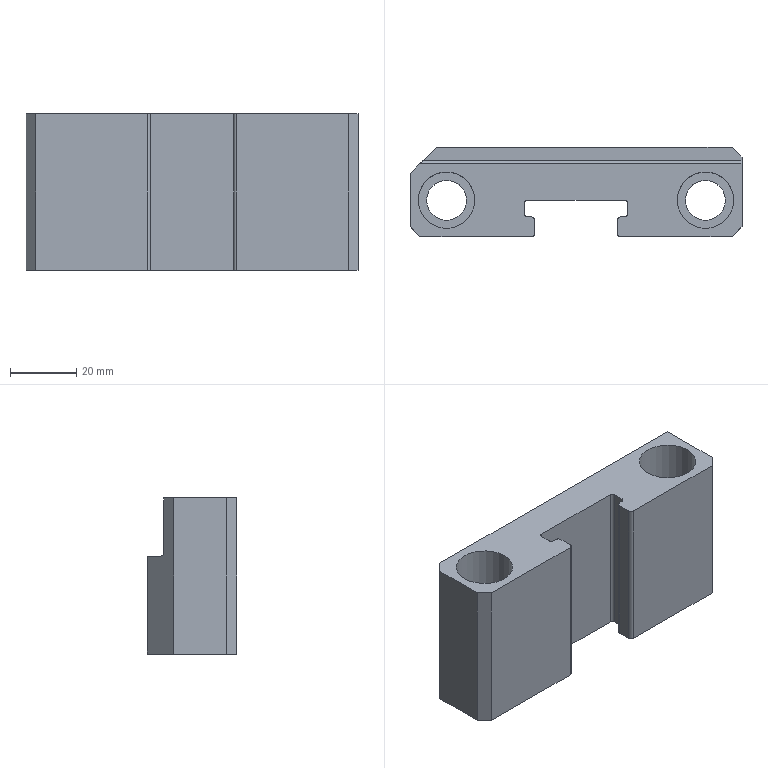Part | NX | features DIE-84 2 | 1 solid | 35 faces | box 100 x 27 x 47 mm | volume 84311 mm3 | plane 22 | cylinder 13 | commonest cylinder face diameters 1.8 x4 2 x3 2.2 x2 12.002 x2 17 x2
STEP:
#1=CARTESIAN_POINT('',(3996.095,-923.622,813.716));
#2=VERTEX_POINT('',#1);
#3=CARTESIAN_POINT('',(3990.094,-923.622,813.716));
#4=DIRECTION('',(0.,0.,1.));
#5=DIRECTION('',(1.,0.,0.));
#6=AXIS2_PLACEMENT_3D('',#3,#4,#5);
#7=CIRCLE('',#6,6.001);
#8=EDGE_CURVE('',#2,#2,#7,.T.);
#9=ORIENTED_EDGE('',*,*,#8,.T.);
#10=EDGE_LOOP('',(#9));
#11=FACE_BOUND('',#10,.T.);
#12=CARTESIAN_POINT('',(3906.093,-923.622,813.716));
#13=VERTEX_POINT('',#12);
#14=CARTESIAN_POINT('',(3912.094,-923.622,813.716));
#15=DIRECTION('',(0.,0.,-1.));
#16=DIRECTION('',(-1.,0.,0.));
#17=AXIS2_PLACEMENT_3D('',#14,#15,#16);
#18=CIRCLE('',#17,6.001);
#19=EDGE_CURVE('',#13,#13,#18,.T.);
#20=ORIENTED_EDGE('',*,*,#19,.F.);
#21=EDGE_LOOP('',(#20));
#22=FACE_BOUND('',#21,.T.);
#23=CARTESIAN_POINT('',(3964.599,-934.622,813.716));
#24=VERTEX_POINT('',#23);
#25=CARTESIAN_POINT('',(3998.094,-934.622,813.716));
#26=VERTEX_POINT('',#25);
#27=CARTESIAN_POINT('',(3911.094,-934.622,813.716));
#28=DIRECTION('',(1.,0.,0.));
#29=VECTOR('',#28,1000.);
#30=LINE('',#27,#29);
#31=EDGE_CURVE('',#24,#26,#30,.T.);
#32=ORIENTED_EDGE('',*,*,#31,.F.);
#33=CARTESIAN_POINT('',(3963.599,-933.622,813.716));
#34=VERTEX_POINT('',#33);
#35=CARTESIAN_POINT('',(3964.599,-933.622,813.716));
#36=DIRECTION('',(0.,0.,-1.));
#37=DIRECTION('',(-1.,0.,0.));
#38=AXIS2_PLACEMENT_3D('',#35,#36,#37);
#39=CIRCLE('',#38,1.);
#40=EDGE_CURVE('',#24,#34,#39,.T.);
#41=ORIENTED_EDGE('',*,*,#40,.T.);
#42=CARTESIAN_POINT('',(3963.599,-929.727,813.716));
#43=VERTEX_POINT('',#42);
#44=CARTESIAN_POINT('',(3963.599,-932.622,813.716));
#45=DIRECTION('',(0.,1.,0.));
#46=VECTOR('',#45,1000.);
#47=LINE('',#44,#46);
#48=EDGE_CURVE('',#34,#43,#47,.T.);
#49=ORIENTED_EDGE('',*,*,#48,.T.);
#50=CARTESIAN_POINT('',(3964.699,-928.627,813.716));
#51=VERTEX_POINT('',#50);
#52=CARTESIAN_POINT('',(3964.699,-929.727,813.716));
#53=DIRECTION('',(0.,0.,-1.));
#54=DIRECTION('',(0.,1.,0.));
#55=AXIS2_PLACEMENT_3D('',#52,#53,#54);
#56=CIRCLE('',#55,1.1);
#57=EDGE_CURVE('',#43,#51,#56,.T.);
#58=ORIENTED_EDGE('',*,*,#57,.T.);
#59=CARTESIAN_POINT('',(3965.699,-928.627,813.716));
#60=VERTEX_POINT('',#59);
#61=CARTESIAN_POINT('',(3964.699,-928.627,813.716));
#62=DIRECTION('',(1.,0.,0.));
#63=VECTOR('',#62,1000.);
#64=LINE('',#61,#63);
#65=EDGE_CURVE('',#51,#60,#64,.T.);
#66=ORIENTED_EDGE('',*,*,#65,.T.);
#67=CARTESIAN_POINT('',(3966.599,-927.727,813.716));
#68=VERTEX_POINT('',#67);
#69=CARTESIAN_POINT('',(3965.699,-927.727,813.716));
#70=DIRECTION('',(0.,0.,1.));
#71=DIRECTION('',(0.,1.,0.));
#72=AXIS2_PLACEMENT_3D('',#69,#70,#71);
#73=CIRCLE('',#72,0.9);
#74=EDGE_CURVE('',#60,#68,#73,.T.);
#75=ORIENTED_EDGE('',*,*,#74,.T.);
#76=CARTESIAN_POINT('',(3966.599,-924.517,813.716));
#77=VERTEX_POINT('',#76);
#78=CARTESIAN_POINT('',(3966.599,-926.727,813.716));
#79=DIRECTION('',(0.,1.,0.));
#80=VECTOR('',#79,1000.);
#81=LINE('',#78,#80);
#82=EDGE_CURVE('',#68,#77,#81,.T.);
#83=ORIENTED_EDGE('',*,*,#82,.T.);
#84=CARTESIAN_POINT('',(3965.699,-923.617,813.716));
#85=VERTEX_POINT('',#84);
#86=CARTESIAN_POINT('',(3965.699,-924.517,813.716));
#87=DIRECTION('',(0.,0.,1.));
#88=DIRECTION('',(0.,1.,0.));
#89=AXIS2_PLACEMENT_3D('',#86,#87,#88);
#90=CIRCLE('',#89,0.9);
#91=EDGE_CURVE('',#77,#85,#90,.T.);
#92=ORIENTED_EDGE('',*,*,#91,.T.);
#93=CARTESIAN_POINT('',(3936.489,-923.617,813.716));
#94=VERTEX_POINT('',#93);
#95=CARTESIAN_POINT('',(3965.699,-923.617,813.716));
#96=DIRECTION('',(-1.,0.,0.));
#97=VECTOR('',#96,1000.);
#98=LINE('',#95,#97);
#99=EDGE_CURVE('',#85,#94,#98,.T.);
#100=ORIENTED_EDGE('',*,*,#99,.T.);
#101=CARTESIAN_POINT('',(3935.589,-924.517,813.716));
#102=VERTEX_POINT('',#101);
#103=CARTESIAN_POINT('',(3936.489,-924.517,813.716));
#104=DIRECTION('',(0.,0.,1.));
#105=DIRECTION('',(0.,1.,0.));
#106=AXIS2_PLACEMENT_3D('',#103,#104,#105);
#107=CIRCLE('',#106,0.9);
#108=EDGE_CURVE('',#94,#102,#107,.T.);
#109=ORIENTED_EDGE('',*,*,#108,.T.);
#110=CARTESIAN_POINT('',(3935.589,-927.727,813.716));
#111=VERTEX_POINT('',#110);
#112=CARTESIAN_POINT('',(3935.589,-924.517,813.716));
#113=DIRECTION('',(0.,-1.,0.));
#114=VECTOR('',#113,1000.);
#115=LINE('',#112,#114);
#116=EDGE_CURVE('',#102,#111,#115,.T.);
#117=ORIENTED_EDGE('',*,*,#116,.T.);
#118=CARTESIAN_POINT('',(3936.489,-928.627,813.716));
#119=VERTEX_POINT('',#118);
#120=CARTESIAN_POINT('',(3936.489,-927.727,813.716));
#121=DIRECTION('',(0.,0.,1.));
#122=DIRECTION('',(0.,1.,0.));
#123=AXIS2_PLACEMENT_3D('',#120,#121,#122);
#124=CIRCLE('',#123,0.9);
#125=EDGE_CURVE('',#111,#119,#124,.T.);
#126=ORIENTED_EDGE('',*,*,#125,.T.);
#127=CARTESIAN_POINT('',(3937.489,-928.627,813.716));
#128=VERTEX_POINT('',#127);
#129=CARTESIAN_POINT('',(3936.489,-928.627,813.716));
#130=DIRECTION('',(1.,0.,0.));
#131=VECTOR('',#130,1000.);
#132=LINE('',#129,#131);
#133=EDGE_CURVE('',#119,#128,#132,.T.);
#134=ORIENTED_EDGE('',*,*,#133,.T.);
#135=CARTESIAN_POINT('',(3938.589,-929.727,813.716));
#136=VERTEX_POINT('',#135);
#137=CARTESIAN_POINT('',(3937.489,-929.727,813.716));
#138=DIRECTION('',(0.,0.,-1.));
#139=DIRECTION('',(0.,1.,0.));
#140=AXIS2_PLACEMENT_3D('',#137,#138,#139);
#141=CIRCLE('',#140,1.1);
#142=EDGE_CURVE('',#128,#136,#141,.T.);
#143=ORIENTED_EDGE('',*,*,#142,.T.);
#144=CARTESIAN_POINT('',(3938.589,-933.622,813.716));
#145=VERTEX_POINT('',#144);
#146=CARTESIAN_POINT('',(3938.589,-928.727,813.716));
#147=DIRECTION('',(0.,-1.,0.));
#148=VECTOR('',#147,1000.);
#149=LINE('',#146,#148);
#150=EDGE_CURVE('',#136,#145,#149,.T.);
#151=ORIENTED_EDGE('',*,*,#150,.T.);
#152=CARTESIAN_POINT('',(3937.589,-934.622,813.716));
#153=VERTEX_POINT('',#152);
#154=CARTESIAN_POINT('',(3937.589,-933.622,813.716));
#155=DIRECTION('',(0.,0.,-1.));
#156=DIRECTION('',(-1.,0.,0.));
#157=AXIS2_PLACEMENT_3D('',#154,#155,#156);
#158=CIRCLE('',#157,1.);
#159=EDGE_CURVE('',#145,#153,#158,.T.);
#160=ORIENTED_EDGE('',*,*,#159,.T.);
#161=CARTESIAN_POINT('',(3904.094,-934.622,813.716));
#162=VERTEX_POINT('',#161);
#163=CARTESIAN_POINT('',(3911.094,-934.622,813.716));
#164=DIRECTION('',(1.,0.,0.));
#165=VECTOR('',#164,1000.);
#166=LINE('',#163,#165);
#167=EDGE_CURVE('',#162,#153,#166,.T.);
#168=ORIENTED_EDGE('',*,*,#167,.F.);
#169=CARTESIAN_POINT('',(3901.094,-931.622,813.716));
#170=VERTEX_POINT('',#169);
#171=CARTESIAN_POINT('',(3901.594,-932.122,813.716));
#172=DIRECTION('',(0.7071,-0.7071,0.));
#173=VECTOR('',#172,1000.);
#174=LINE('',#171,#173);
#175=EDGE_CURVE('',#162,#170,#174,.F.);
#176=ORIENTED_EDGE('',*,*,#175,.T.);
#177=CARTESIAN_POINT('',(3901.094,-915.622,813.716));
#178=VERTEX_POINT('',#177);
#179=CARTESIAN_POINT('',(3901.094,-922.622,813.716));
#180=DIRECTION('',(0.,-1.,0.));
#181=VECTOR('',#180,1000.);
#182=LINE('',#179,#181);
#183=EDGE_CURVE('',#178,#170,#182,.T.);
#184=ORIENTED_EDGE('',*,*,#183,.F.);
#185=CARTESIAN_POINT('',(3909.094,-907.622,813.716));
#186=VERTEX_POINT('',#185);
#187=CARTESIAN_POINT('',(3905.094,-911.622,813.716));
#188=DIRECTION('',(-0.7071,-0.7071,0.));
#189=VECTOR('',#188,1000.);
#190=LINE('',#187,#189);
#191=EDGE_CURVE('',#178,#186,#190,.F.);
#192=ORIENTED_EDGE('',*,*,#191,.T.);
#193=CARTESIAN_POINT('',(3998.094,-907.622,813.716));
#194=VERTEX_POINT('',#193);
#195=CARTESIAN_POINT('',(3911.094,-907.622,813.716));
#196=DIRECTION('',(-1.,0.,0.));
#197=VECTOR('',#196,1000.);
#198=LINE('',#195,#197);
#199=EDGE_CURVE('',#194,#186,#198,.T.);
#200=ORIENTED_EDGE('',*,*,#199,.F.);
#201=CARTESIAN_POINT('',(4001.094,-910.622,813.716));
#202=VERTEX_POINT('',#201);
#203=CARTESIAN_POINT('',(3962.094,-871.622,813.716));
#204=DIRECTION('',(-0.7071,0.7071,0.));
#205=VECTOR('',#204,1000.);
#206=LINE('',#203,#205);
#207=EDGE_CURVE('',#194,#202,#206,.F.);
#208=ORIENTED_EDGE('',*,*,#207,.T.);
#209=CARTESIAN_POINT('',(4001.094,-931.622,813.716));
#210=VERTEX_POINT('',#209);
#211=CARTESIAN_POINT('',(4001.094,-922.622,813.716));
#212=DIRECTION('',(0.,1.,0.));
#213=VECTOR('',#212,1000.);
#214=LINE('',#211,#213);
#215=EDGE_CURVE('',#210,#202,#214,.T.);
#216=ORIENTED_EDGE('',*,*,#215,.F.);
#217=CARTESIAN_POINT('',(3960.594,-972.122,813.716));
#218=DIRECTION('',(0.7071,0.7071,0.));
#219=VECTOR('',#218,1000.);
#220=LINE('',#217,#219);
#221=EDGE_CURVE('',#210,#26,#220,.F.);
#222=ORIENTED_EDGE('',*,*,#221,.T.);
#223=EDGE_LOOP('',(#32,#41,#49,#58,#66,#75,#83,#92,#100,#109,#117,#126,#134,#143,#151,#160,#168,#176,#184,#192,#200,#208,#216,#222));
#224=FACE_BOUND('',#223,.T.);
#225=CARTESIAN_POINT('',(3911.094,-922.622,813.716));
#226=DIRECTION('',(0.,0.,-1.));
#227=DIRECTION('',(-1.,0.,0.));
#228=AXIS2_PLACEMENT_3D('',#225,#226,#227);
#229=PLANE('',#228);
#230=ADVANCED_FACE('',(#11,#22,#224),#229,.T.);
#231=CARTESIAN_POINT('',(3998.094,-934.622,860.716));
#232=VERTEX_POINT('',#231);
#233=CARTESIAN_POINT('',(4001.094,-931.622,860.716));
#234=VERTEX_POINT('',#233);
#235=CARTESIAN_POINT('',(3960.594,-972.122,860.716));
#236=DIRECTION('',(-0.7071,-0.7071,0.));
#237=VECTOR('',#236,1000.);
#238=LINE('',#235,#237);
#239=EDGE_CURVE('',#232,#234,#238,.F.);
#240=ORIENTED_EDGE('',*,*,#239,.F.);
#241=CARTESIAN_POINT('',(3998.094,-934.622,821.716));
#242=DIRECTION('',(0.,0.,-1.));
#243=VECTOR('',#242,1000.);
#244=LINE('',#241,#243);
#245=EDGE_CURVE('',#26,#232,#244,.F.);
#246=ORIENTED_EDGE('',*,*,#245,.F.);
#247=ORIENTED_EDGE('',*,*,#221,.F.);
#248=CARTESIAN_POINT('',(4001.094,-931.622,821.716));
#249=DIRECTION('',(0.,0.,1.));
#250=VECTOR('',#249,1000.);
#251=LINE('',#248,#250);
#252=EDGE_CURVE('',#234,#210,#251,.F.);
#253=ORIENTED_EDGE('',*,*,#252,.F.);
#254=EDGE_LOOP('',(#240,#246,#247,#253));
#255=FACE_BOUND('',#254,.T.);
#256=CARTESIAN_POINT('',(3998.094,-934.622,821.716));
#257=DIRECTION('',(-0.7071,0.7071,0.));
#258=DIRECTION('',(-0.7071,-0.7071,0.));
#259=AXIS2_PLACEMENT_3D('',#256,#257,#258);
#260=PLANE('',#259);
#261=ADVANCED_FACE('',(#255),#260,.F.);
#262=CARTESIAN_POINT('',(3998.094,-907.622,843.216));
#263=VERTEX_POINT('',#262);
#264=CARTESIAN_POINT('',(3998.094,-907.622,821.716));
#265=DIRECTION('',(0.,0.,1.));
#266=VECTOR('',#265,1000.);
#267=LINE('',#264,#266);
#268=EDGE_CURVE('',#263,#194,#267,.F.);
#269=ORIENTED_EDGE('',*,*,#268,.F.);
#270=CARTESIAN_POINT('',(4001.094,-910.622,843.216));
#271=VERTEX_POINT('',#270);
#272=CARTESIAN_POINT('',(4001.094,-910.622,843.216));
#273=DIRECTION('',(0.7071,-0.7071,0.));
#274=VECTOR('',#273,1000.);
#275=LINE('',#272,#274);
#276=EDGE_CURVE('',#271,#263,#275,.F.);
#277=ORIENTED_EDGE('',*,*,#276,.F.);
#278=CARTESIAN_POINT('',(4001.094,-910.622,821.716));
#279=DIRECTION('',(0.,0.,-1.));
#280=VECTOR('',#279,1000.);
#281=LINE('',#278,#280);
#282=EDGE_CURVE('',#202,#271,#281,.F.);
#283=ORIENTED_EDGE('',*,*,#282,.F.);
#284=ORIENTED_EDGE('',*,*,#207,.F.);
#285=EDGE_LOOP('',(#269,#277,#283,#284));
#286=FACE_BOUND('',#285,.T.);
#287=CARTESIAN_POINT('',(4001.094,-910.622,821.716));
#288=DIRECTION('',(-0.7071,-0.7071,0.));
#289=DIRECTION('',(0.7071,-0.7071,0.));
#290=AXIS2_PLACEMENT_3D('',#287,#288,#289);
#291=PLANE('',#290);
#292=ADVANCED_FACE('',(#286),#291,.F.);
#293=ORIENTED_EDGE('',*,*,#282,.T.);
#294=CARTESIAN_POINT('',(4001.094,-911.622,843.216));
#295=VERTEX_POINT('',#294);
#296=CARTESIAN_POINT('',(4001.094,-922.622,843.216));
#297=DIRECTION('',(0.,-1.,0.));
#298=VECTOR('',#297,1000.);
#299=LINE('',#296,#298);
#300=EDGE_CURVE('',#271,#295,#299,.T.);
#301=ORIENTED_EDGE('',*,*,#300,.T.);
#302=CARTESIAN_POINT('',(4001.094,-912.622,844.216));
#303=VERTEX_POINT('',#302);
#304=CARTESIAN_POINT('',(4001.094,-911.622,844.216));
#305=DIRECTION('',(1.,0.,0.));
#306=DIRECTION('',(0.,0.,-1.));
#307=AXIS2_PLACEMENT_3D('',#304,#305,#306);
#308=CIRCLE('',#307,1.);
#309=EDGE_CURVE('',#295,#303,#308,.F.);
#310=ORIENTED_EDGE('',*,*,#309,.T.);
#311=CARTESIAN_POINT('',(4001.094,-912.622,860.716));
#312=VERTEX_POINT('',#311);
#313=CARTESIAN_POINT('',(4001.094,-912.622,821.716));
#314=DIRECTION('',(0.,0.,-1.));
#315=VECTOR('',#314,1000.);
#316=LINE('',#313,#315);
#317=EDGE_CURVE('',#312,#303,#316,.T.);
#318=ORIENTED_EDGE('',*,*,#317,.F.);
#319=CARTESIAN_POINT('',(4001.094,-922.622,860.716));
#320=DIRECTION('',(0.,-1.,0.));
#321=VECTOR('',#320,1000.);
#322=LINE('',#319,#321);
#323=EDGE_CURVE('',#312,#234,#322,.T.);
#324=ORIENTED_EDGE('',*,*,#323,.T.);
#325=ORIENTED_EDGE('',*,*,#252,.T.);
#326=ORIENTED_EDGE('',*,*,#215,.T.);
#327=EDGE_LOOP('',(#293,#301,#310,#318,#324,#325,#326));
#328=FACE_BOUND('',#327,.T.);
#329=CARTESIAN_POINT('',(4001.094,-922.622,821.716));
#330=DIRECTION('',(1.,0.,0.));
#331=DIRECTION('',(0.,0.,-1.));
#332=AXIS2_PLACEMENT_3D('',#329,#330,#331);
#333=PLANE('',#332);
#334=ADVANCED_FACE('',(#328),#333,.T.);
#335=CARTESIAN_POINT('',(3901.094,-915.622,860.716));
#336=VERTEX_POINT('',#335);
#337=CARTESIAN_POINT('',(3901.094,-915.622,821.716));
#338=DIRECTION('',(0.,0.,-1.));
#339=VECTOR('',#338,1000.);
#340=LINE('',#337,#339);
#341=EDGE_CURVE('',#336,#178,#340,.T.);
#342=ORIENTED_EDGE('',*,*,#341,.F.);
#343=CARTESIAN_POINT('',(3904.094,-912.622,860.716));
#344=VERTEX_POINT('',#343);
#345=CARTESIAN_POINT('',(3902.594,-914.122,860.716));
#346=DIRECTION('',(0.7071,0.7071,0.));
#347=VECTOR('',#346,1000.);
#348=LINE('',#345,#347);
#349=EDGE_CURVE('',#344,#336,#348,.F.);
#350=ORIENTED_EDGE('',*,*,#349,.F.);
#351=CARTESIAN_POINT('',(3904.094,-912.622,844.216));
#352=VERTEX_POINT('',#351);
#353=CARTESIAN_POINT('',(3904.094,-912.622,821.716));
#354=DIRECTION('',(0.,0.,-1.));
#355=VECTOR('',#354,1000.);
#356=LINE('',#353,#355);
#357=EDGE_CURVE('',#352,#344,#356,.F.);
#358=ORIENTED_EDGE('',*,*,#357,.F.);
#359=CARTESIAN_POINT('',(3905.094,-911.622,843.216));
#360=VERTEX_POINT('',#359);
#361=CARTESIAN_POINT('',(3905.094,-911.622,844.216));
#362=DIRECTION('',(0.7071,-0.7071,0.));
#363=DIRECTION('',(-0.7071,-0.7071,0.));
#364=AXIS2_PLACEMENT_3D('',#361,#362,#363);
#365=ELLIPSE('',#364,1.414,1.);
#366=EDGE_CURVE('',#352,#360,#365,.T.);
#367=ORIENTED_EDGE('',*,*,#366,.T.);
#368=CARTESIAN_POINT('',(3909.094,-907.622,843.216));
#369=VERTEX_POINT('',#368);
#370=CARTESIAN_POINT('',(3909.094,-907.622,843.216));
#371=DIRECTION('',(0.7071,0.7071,0.));
#372=VECTOR('',#371,1000.);
#373=LINE('',#370,#372);
#374=EDGE_CURVE('',#369,#360,#373,.F.);
#375=ORIENTED_EDGE('',*,*,#374,.F.);
#376=CARTESIAN_POINT('',(3909.094,-907.622,821.716));
#377=DIRECTION('',(0.,0.,1.));
#378=VECTOR('',#377,1000.);
#379=LINE('',#376,#378);
#380=EDGE_CURVE('',#186,#369,#379,.T.);
#381=ORIENTED_EDGE('',*,*,#380,.F.);
#382=ORIENTED_EDGE('',*,*,#191,.F.);
#383=EDGE_LOOP('',(#342,#350,#358,#367,#375,#381,#382));
#384=FACE_BOUND('',#383,.T.);
#385=CARTESIAN_POINT('',(3909.094,-907.622,821.716));
#386=DIRECTION('',(0.7071,-0.7071,0.));
#387=DIRECTION('',(0.,0.,1.));
#388=AXIS2_PLACEMENT_3D('',#385,#386,#387);
#389=PLANE('',#388);
#390=ADVANCED_FACE('',(#384),#389,.F.);
#391=ORIENTED_EDGE('',*,*,#380,.T.);
#392=CARTESIAN_POINT('',(3946.094,-907.622,843.216));
#393=DIRECTION('',(1.,0.,0.));
#394=VECTOR('',#393,1000.);
#395=LINE('',#392,#394);
#396=EDGE_CURVE('',#369,#263,#395,.T.);
#397=ORIENTED_EDGE('',*,*,#396,.T.);
#398=ORIENTED_EDGE('',*,*,#268,.T.);
#399=ORIENTED_EDGE('',*,*,#199,.T.);
#400=EDGE_LOOP('',(#391,#397,#398,#399));
#401=FACE_BOUND('',#400,.T.);
#402=CARTESIAN_POINT('',(3911.094,-907.622,821.716));
#403=DIRECTION('',(0.,1.,0.));
#404=DIRECTION('',(0.,0.,1.));
#405=AXIS2_PLACEMENT_3D('',#402,#403,#404);
#406=PLANE('',#405);
#407=ADVANCED_FACE('',(#401),#406,.T.);
#408=CARTESIAN_POINT('',(3904.094,-934.622,860.716));
#409=VERTEX_POINT('',#408);
#410=CARTESIAN_POINT('',(3904.094,-934.622,821.716));
#411=DIRECTION('',(0.,0.,1.));
#412=VECTOR('',#411,1000.);
#413=LINE('',#410,#412);
#414=EDGE_CURVE('',#409,#162,#413,.F.);
#415=ORIENTED_EDGE('',*,*,#414,.F.);
#416=CARTESIAN_POINT('',(3901.094,-931.622,860.716));
#417=VERTEX_POINT('',#416);
#418=CARTESIAN_POINT('',(3901.594,-932.122,860.716));
#419=DIRECTION('',(-0.7071,0.7071,0.));
#420=VECTOR('',#419,1000.);
#421=LINE('',#418,#420);
#422=EDGE_CURVE('',#417,#409,#421,.F.);
#423=ORIENTED_EDGE('',*,*,#422,.F.);
#424=CARTESIAN_POINT('',(3901.094,-931.622,821.716));
#425=DIRECTION('',(0.,0.,-1.));
#426=VECTOR('',#425,1000.);
#427=LINE('',#424,#426);
#428=EDGE_CURVE('',#170,#417,#427,.F.);
#429=ORIENTED_EDGE('',*,*,#428,.F.);
#430=ORIENTED_EDGE('',*,*,#175,.F.);
#431=EDGE_LOOP('',(#415,#423,#429,#430));
#432=FACE_BOUND('',#431,.T.);
#433=CARTESIAN_POINT('',(3901.094,-931.622,821.716));
#434=DIRECTION('',(0.7071,0.7071,0.));
#435=DIRECTION('',(-0.7071,0.7071,0.));
#436=AXIS2_PLACEMENT_3D('',#433,#434,#435);
#437=PLANE('',#436);
#438=ADVANCED_FACE('',(#432),#437,.F.);
#439=ORIENTED_EDGE('',*,*,#428,.T.);
#440=CARTESIAN_POINT('',(3901.094,-922.622,860.716));
#441=DIRECTION('',(0.,1.,0.));
#442=VECTOR('',#441,1000.);
#443=LINE('',#440,#442);
#444=EDGE_CURVE('',#417,#336,#443,.T.);
#445=ORIENTED_EDGE('',*,*,#444,.T.);
#446=ORIENTED_EDGE('',*,*,#341,.T.);
#447=ORIENTED_EDGE('',*,*,#183,.T.);
#448=EDGE_LOOP('',(#439,#445,#446,#447));
#449=FACE_BOUND('',#448,.T.);
#450=CARTESIAN_POINT('',(3901.094,-922.622,821.716));
#451=DIRECTION('',(-1.,0.,0.));
#452=DIRECTION('',(0.,0.,1.));
#453=AXIS2_PLACEMENT_3D('',#450,#451,#452);
#454=PLANE('',#453);
#455=ADVANCED_FACE('',(#449),#454,.T.);
#456=CARTESIAN_POINT('',(3964.599,-934.622,860.716));
#457=VERTEX_POINT('',#456);
#458=CARTESIAN_POINT('',(3964.599,-934.622,813.716));
#459=DIRECTION('',(0.,0.,1.));
#460=VECTOR('',#459,1000.);
#461=LINE('',#458,#460);
#462=EDGE_CURVE('',#457,#24,#461,.F.);
#463=ORIENTED_EDGE('',*,*,#462,.F.);
#464=CARTESIAN_POINT('',(3963.599,-933.622,860.716));
#465=VERTEX_POINT('',#464);
#466=CARTESIAN_POINT('',(3964.599,-933.622,860.716));
#467=DIRECTION('',(0.,0.,1.));
#468=DIRECTION('',(1.,0.,0.));
#469=AXIS2_PLACEMENT_3D('',#466,#467,#468);
#470=CIRCLE('',#469,1.);
#471=EDGE_CURVE('',#457,#465,#470,.F.);
#472=ORIENTED_EDGE('',*,*,#471,.T.);
#473=CARTESIAN_POINT('',(3963.599,-933.622,859.716));
#474=DIRECTION('',(0.,0.,1.));
#475=VECTOR('',#474,1000.);
#476=LINE('',#473,#475);
#477=EDGE_CURVE('',#34,#465,#476,.T.);
#478=ORIENTED_EDGE('',*,*,#477,.F.);
#479=ORIENTED_EDGE('',*,*,#40,.F.);
#480=EDGE_LOOP('',(#463,#472,#478,#479));
#481=FACE_BOUND('',#480,.T.);
#482=CARTESIAN_POINT('',(3964.599,-933.622,813.716));
#483=DIRECTION('',(0.,0.,-1.));
#484=DIRECTION('',(-1.,0.,0.));
#485=AXIS2_PLACEMENT_3D('',#482,#483,#484);
#486=CYLINDRICAL_SURFACE('',#485,1.);
#487=ADVANCED_FACE('',(#481),#486,.T.);
#488=CARTESIAN_POINT('',(3938.589,-933.622,860.716));
#489=VERTEX_POINT('',#488);
#490=CARTESIAN_POINT('',(3938.589,-933.622,813.716));
#491=DIRECTION('',(0.,0.,-1.));
#492=VECTOR('',#491,1000.);
#493=LINE('',#490,#492);
#494=EDGE_CURVE('',#489,#145,#493,.T.);
#495=ORIENTED_EDGE('',*,*,#494,.F.);
#496=CARTESIAN_POINT('',(3937.589,-934.622,860.716));
#497=VERTEX_POINT('',#496);
#498=CARTESIAN_POINT('',(3937.589,-933.622,860.716));
#499=DIRECTION('',(0.,0.,1.));
#500=DIRECTION('',(1.,0.,0.));
#501=AXIS2_PLACEMENT_3D('',#498,#499,#500);
#502=CIRCLE('',#501,1.);
#503=EDGE_CURVE('',#489,#497,#502,.F.);
#504=ORIENTED_EDGE('',*,*,#503,.T.);
#505=CARTESIAN_POINT('',(3937.589,-934.622,859.716));
#506=DIRECTION('',(0.,0.,-1.));
#507=VECTOR('',#506,1000.);
#508=LINE('',#505,#507);
#509=EDGE_CURVE('',#153,#497,#508,.F.);
#510=ORIENTED_EDGE('',*,*,#509,.F.);
#511=ORIENTED_EDGE('',*,*,#159,.F.);
#512=EDGE_LOOP('',(#495,#504,#510,#511));
#513=FACE_BOUND('',#512,.T.);
#514=CARTESIAN_POINT('',(3937.589,-933.622,813.716));
#515=DIRECTION('',(0.,0.,1.));
#516=DIRECTION('',(1.,0.,0.));
#517=AXIS2_PLACEMENT_3D('',#514,#515,#516);
#518=CYLINDRICAL_SURFACE('',#517,1.);
#519=ADVANCED_FACE('',(#513),#518,.T.);
#520=CARTESIAN_POINT('',(3938.589,-929.727,860.716));
#521=VERTEX_POINT('',#520);
#522=CARTESIAN_POINT('',(3938.589,-922.622,860.716));
#523=DIRECTION('',(0.,-1.,0.));
#524=VECTOR('',#523,1000.);
#525=LINE('',#522,#524);
#526=EDGE_CURVE('',#521,#489,#525,.T.);
#527=ORIENTED_EDGE('',*,*,#526,.T.);
#528=ORIENTED_EDGE('',*,*,#494,.T.);
#529=ORIENTED_EDGE('',*,*,#150,.F.);
#530=CARTESIAN_POINT('',(3938.589,-929.727,813.716));
#531=DIRECTION('',(0.,0.,1.));
#532=VECTOR('',#531,1000.);
#533=LINE('',#530,#532);
#534=EDGE_CURVE('',#136,#521,#533,.T.);
#535=ORIENTED_EDGE('',*,*,#534,.T.);
#536=EDGE_LOOP('',(#527,#528,#529,#535));
#537=FACE_BOUND('',#536,.T.);
#538=CARTESIAN_POINT('',(3938.589,-928.727,813.716));
#539=DIRECTION('',(-1.,0.,0.));
#540=DIRECTION('',(0.,0.,1.));
#541=AXIS2_PLACEMENT_3D('',#538,#539,#540);
#542=PLANE('',#541);
#543=ADVANCED_FACE('',(#537),#542,.F.);
#544=CARTESIAN_POINT('',(3937.489,-928.627,860.716));
#545=VERTEX_POINT('',#544);
#546=CARTESIAN_POINT('',(3937.489,-928.627,813.716));
#547=DIRECTION('',(0.,0.,1.));
#548=VECTOR('',#547,1000.);
#549=LINE('',#546,#548);
#550=EDGE_CURVE('',#128,#545,#549,.T.);
#551=ORIENTED_EDGE('',*,*,#550,.T.);
#552=CARTESIAN_POINT('',(3937.489,-929.727,860.716));
#553=DIRECTION('',(0.,0.,1.));
#554=DIRECTION('',(1.,0.,0.));
#555=AXIS2_PLACEMENT_3D('',#552,#553,#554);
#556=CIRCLE('',#555,1.1);
#557=EDGE_CURVE('',#545,#521,#556,.F.);
#558=ORIENTED_EDGE('',*,*,#557,.T.);
#559=ORIENTED_EDGE('',*,*,#534,.F.);
#560=ORIENTED_EDGE('',*,*,#142,.F.);
#561=EDGE_LOOP('',(#551,#558,#559,#560));
#562=FACE_BOUND('',#561,.T.);
#563=CARTESIAN_POINT('',(3937.489,-929.727,813.716));
#564=DIRECTION('',(0.,0.,1.));
#565=DIRECTION('',(1.,0.,0.));
#566=AXIS2_PLACEMENT_3D('',#563,#564,#565);
#567=CYLINDRICAL_SURFACE('',#566,1.1);
#568=ADVANCED_FACE('',(#562),#567,.T.);
#569=CARTESIAN_POINT('',(3936.489,-928.627,860.716));
#570=VERTEX_POINT('',#569);
#571=CARTESIAN_POINT('',(3936.489,-928.627,813.716));
#572=DIRECTION('',(0.,0.,1.));
#573=VECTOR('',#572,1000.);
#574=LINE('',#571,#573);
#575=EDGE_CURVE('',#119,#570,#574,.T.);
#576=ORIENTED_EDGE('',*,*,#575,.T.);
#577=CARTESIAN_POINT('',(3913.594,-928.627,860.716));
#578=DIRECTION('',(1.,0.,0.));
#579=VECTOR('',#578,1000.);
#580=LINE('',#577,#579);
#581=EDGE_CURVE('',#570,#545,#580,.T.);
#582=ORIENTED_EDGE('',*,*,#581,.T.);
#583=ORIENTED_EDGE('',*,*,#550,.F.);
#584=ORIENTED_EDGE('',*,*,#133,.F.);
#585=EDGE_LOOP('',(#576,#582,#583,#584));
#586=FACE_BOUND('',#585,.T.);
#587=CARTESIAN_POINT('',(3936.489,-928.627,813.716));
#588=DIRECTION('',(0.,-1.,0.));
#589=DIRECTION('',(0.,0.,-1.));
#590=AXIS2_PLACEMENT_3D('',#587,#588,#589);
#591=PLANE('',#590);
#592=ADVANCED_FACE('',(#586),#591,.F.);
#593=CARTESIAN_POINT('',(3935.589,-927.727,860.716));
#594=VERTEX_POINT('',#593);
#595=CARTESIAN_POINT('',(3935.589,-927.727,813.716));
#596=DIRECTION('',(0.,0.,1.));
#597=VECTOR('',#596,1000.);
#598=LINE('',#595,#597);
#599=EDGE_CURVE('',#111,#594,#598,.T.);
#600=ORIENTED_EDGE('',*,*,#599,.T.);
#601=CARTESIAN_POINT('',(3936.489,-927.727,860.716));
#602=DIRECTION('',(0.,0.,1.));
#603=DIRECTION('',(1.,0.,0.));
#604=AXIS2_PLACEMENT_3D('',#601,#602,#603);
#605=CIRCLE('',#604,0.9);
#606=EDGE_CURVE('',#594,#570,#605,.T.);
#607=ORIENTED_EDGE('',*,*,#606,.T.);
#608=ORIENTED_EDGE('',*,*,#575,.F.);
#609=ORIENTED_EDGE('',*,*,#125,.F.);
#610=EDGE_LOOP('',(#600,#607,#608,#609));
#611=FACE_BOUND('',#610,.T.);
#612=CARTESIAN_POINT('',(3936.489,-927.727,813.716));
#613=DIRECTION('',(0.,0.,1.));
#614=DIRECTION('',(1.,0.,0.));
#615=AXIS2_PLACEMENT_3D('',#612,#613,#614);
#616=CYLINDRICAL_SURFACE('',#615,0.9);
#617=ADVANCED_FACE('',(#611),#616,.F.);
#618=CARTESIAN_POINT('',(3935.589,-924.517,860.716));
#619=VERTEX_POINT('',#618);
#620=CARTESIAN_POINT('',(3935.589,-924.517,813.716));
#621=DIRECTION('',(0.,0.,1.));
#622=VECTOR('',#621,1000.);
#623=LINE('',#620,#622);
#624=EDGE_CURVE('',#102,#619,#623,.T.);
#625=ORIENTED_EDGE('',*,*,#624,.T.);
#626=CARTESIAN_POINT('',(3935.589,-922.622,860.716));
#627=DIRECTION('',(0.,-1.,0.));
#628=VECTOR('',#627,1000.);
#629=LINE('',#626,#628);
#630=EDGE_CURVE('',#619,#594,#629,.T.);
#631=ORIENTED_EDGE('',*,*,#630,.T.);
#632=ORIENTED_EDGE('',*,*,#599,.F.);
#633=ORIENTED_EDGE('',*,*,#116,.F.);
#634=EDGE_LOOP('',(#625,#631,#632,#633));
#635=FACE_BOUND('',#634,.T.);
#636=CARTESIAN_POINT('',(3935.589,-924.517,813.716));
#637=DIRECTION('',(-1.,0.,0.));
#638=DIRECTION('',(0.,0.,1.));
#639=AXIS2_PLACEMENT_3D('',#636,#637,#638);
#640=PLANE('',#639);
#641=ADVANCED_FACE('',(#635),#640,.F.);
#642=CARTESIAN_POINT('',(3936.489,-923.617,860.716));
#643=VERTEX_POINT('',#642);
#644=CARTESIAN_POINT('',(3936.489,-923.617,813.716));
#645=DIRECTION('',(0.,0.,1.));
#646=VECTOR('',#645,1000.);
#647=LINE('',#644,#646);
#648=EDGE_CURVE('',#94,#643,#647,.T.);
#649=ORIENTED_EDGE('',*,*,#648,.T.);
#650=CARTESIAN_POINT('',(3936.489,-924.517,860.716));
#651=DIRECTION('',(0.,0.,1.));
#652=DIRECTION('',(1.,0.,0.));
#653=AXIS2_PLACEMENT_3D('',#650,#651,#652);
#654=CIRCLE('',#653,0.9);
#655=EDGE_CURVE('',#643,#619,#654,.T.);
#656=ORIENTED_EDGE('',*,*,#655,.T.);
#657=ORIENTED_EDGE('',*,*,#624,.F.);
#658=ORIENTED_EDGE('',*,*,#108,.F.);
#659=EDGE_LOOP('',(#649,#656,#657,#658));
#660=FACE_BOUND('',#659,.T.);
#661=CARTESIAN_POINT('',(3936.489,-924.517,813.716));
#662=DIRECTION('',(0.,0.,1.));
#663=DIRECTION('',(1.,0.,0.));
#664=AXIS2_PLACEMENT_3D('',#661,#662,#663);
#665=CYLINDRICAL_SURFACE('',#664,0.9);
#666=ADVANCED_FACE('',(#660),#665,.F.);
#667=CARTESIAN_POINT('',(3965.699,-923.617,860.716));
#668=VERTEX_POINT('',#667);
#669=CARTESIAN_POINT('',(3965.699,-923.617,813.716));
#670=DIRECTION('',(0.,0.,1.));
#671=VECTOR('',#670,1000.);
#672=LINE('',#669,#671);
#673=EDGE_CURVE('',#85,#668,#672,.T.);
#674=ORIENTED_EDGE('',*,*,#673,.T.);
#675=CARTESIAN_POINT('',(3913.594,-923.617,860.716));
#676=DIRECTION('',(-1.,0.,0.));
#677=VECTOR('',#676,1000.);
#678=LINE('',#675,#677);
#679=EDGE_CURVE('',#668,#643,#678,.T.);
#680=ORIENTED_EDGE('',*,*,#679,.T.);
#681=ORIENTED_EDGE('',*,*,#648,.F.);
#682=ORIENTED_EDGE('',*,*,#99,.F.);
#683=EDGE_LOOP('',(#674,#680,#681,#682));
#684=FACE_BOUND('',#683,.T.);
#685=CARTESIAN_POINT('',(3965.699,-923.617,813.716));
#686=DIRECTION('',(0.,1.,0.));
#687=DIRECTION('',(0.,0.,1.));
#688=AXIS2_PLACEMENT_3D('',#685,#686,#687);
#689=PLANE('',#688);
#690=ADVANCED_FACE('',(#684),#689,.F.);
#691=CARTESIAN_POINT('',(3966.599,-924.517,860.716));
#692=VERTEX_POINT('',#691);
#693=CARTESIAN_POINT('',(3966.599,-924.517,813.716));
#694=DIRECTION('',(0.,0.,1.));
#695=VECTOR('',#694,1000.);
#696=LINE('',#693,#695);
#697=EDGE_CURVE('',#77,#692,#696,.T.);
#698=ORIENTED_EDGE('',*,*,#697,.T.);
#699=CARTESIAN_POINT('',(3965.699,-924.517,860.716));
#700=DIRECTION('',(0.,0.,1.));
#701=DIRECTION('',(1.,0.,0.));
#702=AXIS2_PLACEMENT_3D('',#699,#700,#701);
#703=CIRCLE('',#702,0.9);
#704=EDGE_CURVE('',#692,#668,#703,.T.);
#705=ORIENTED_EDGE('',*,*,#704,.T.);
#706=ORIENTED_EDGE('',*,*,#673,.F.);
#707=ORIENTED_EDGE('',*,*,#91,.F.);
#708=EDGE_LOOP('',(#698,#705,#706,#707));
#709=FACE_BOUND('',#708,.T.);
#710=CARTESIAN_POINT('',(3965.699,-924.517,813.716));
#711=DIRECTION('',(0.,0.,1.));
#712=DIRECTION('',(1.,0.,0.));
#713=AXIS2_PLACEMENT_3D('',#710,#711,#712);
#714=CYLINDRICAL_SURFACE('',#713,0.9);
#715=ADVANCED_FACE('',(#709),#714,.F.);
#716=CARTESIAN_POINT('',(3966.599,-927.727,860.716));
#717=VERTEX_POINT('',#716);
#718=CARTESIAN_POINT('',(3966.599,-927.727,813.716));
#719=DIRECTION('',(0.,0.,1.));
#720=VECTOR('',#719,1000.);
#721=LINE('',#718,#720);
#722=EDGE_CURVE('',#68,#717,#721,.T.);
#723=ORIENTED_EDGE('',*,*,#722,.T.);
#724=CARTESIAN_POINT('',(3966.599,-922.622,860.716));
#725=DIRECTION('',(0.,1.,0.));
#726=VECTOR('',#725,1000.);
#727=LINE('',#724,#726);
#728=EDGE_CURVE('',#717,#692,#727,.T.);
#729=ORIENTED_EDGE('',*,*,#728,.T.);
#730=ORIENTED_EDGE('',*,*,#697,.F.);
#731=ORIENTED_EDGE('',*,*,#82,.F.);
#732=EDGE_LOOP('',(#723,#729,#730,#731));
#733=FACE_BOUND('',#732,.T.);
#734=CARTESIAN_POINT('',(3966.599,-926.727,813.716));
#735=DIRECTION('',(1.,0.,0.));
#736=DIRECTION('',(0.,0.,-1.));
#737=AXIS2_PLACEMENT_3D('',#734,#735,#736);
#738=PLANE('',#737);
#739=ADVANCED_FACE('',(#733),#738,.F.);
#740=CARTESIAN_POINT('',(3965.699,-928.627,860.716));
#741=VERTEX_POINT('',#740);
#742=CARTESIAN_POINT('',(3965.699,-928.627,813.716));
#743=DIRECTION('',(0.,0.,1.));
#744=VECTOR('',#743,1000.);
#745=LINE('',#742,#744);
#746=EDGE_CURVE('',#60,#741,#745,.T.);
#747=ORIENTED_EDGE('',*,*,#746,.T.);
#748=CARTESIAN_POINT('',(3965.699,-927.727,860.716));
#749=DIRECTION('',(0.,0.,1.));
#750=DIRECTION('',(1.,0.,0.));
#751=AXIS2_PLACEMENT_3D('',#748,#749,#750);
#752=CIRCLE('',#751,0.9);
#753=EDGE_CURVE('',#741,#717,#752,.T.);
#754=ORIENTED_EDGE('',*,*,#753,.T.);
#755=ORIENTED_EDGE('',*,*,#722,.F.);
#756=ORIENTED_EDGE('',*,*,#74,.F.);
#757=EDGE_LOOP('',(#747,#754,#755,#756));
#758=FACE_BOUND('',#757,.T.);
#759=CARTESIAN_POINT('',(3965.699,-927.727,813.716));
#760=DIRECTION('',(0.,0.,1.));
#761=DIRECTION('',(1.,0.,0.));
#762=AXIS2_PLACEMENT_3D('',#759,#760,#761);
#763=CYLINDRICAL_SURFACE('',#762,0.9);
#764=ADVANCED_FACE('',(#758),#763,.F.);
#765=CARTESIAN_POINT('',(3964.699,-928.627,860.716));
#766=VERTEX_POINT('',#765);
#767=CARTESIAN_POINT('',(3964.699,-928.627,813.716));
#768=DIRECTION('',(0.,0.,1.));
#769=VECTOR('',#768,1000.);
#770=LINE('',#767,#769);
#771=EDGE_CURVE('',#51,#766,#770,.T.);
#772=ORIENTED_EDGE('',*,*,#771,.T.);
#773=CARTESIAN_POINT('',(3913.594,-928.627,860.716));
#774=DIRECTION('',(1.,0.,0.));
#775=VECTOR('',#774,1000.);
#776=LINE('',#773,#775);
#777=EDGE_CURVE('',#766,#741,#776,.T.);
#778=ORIENTED_EDGE('',*,*,#777,.T.);
#779=ORIENTED_EDGE('',*,*,#746,.F.);
#780=ORIENTED_EDGE('',*,*,#65,.F.);
#781=EDGE_LOOP('',(#772,#778,#779,#780));
#782=FACE_BOUND('',#781,.T.);
#783=CARTESIAN_POINT('',(3964.699,-928.627,813.716));
#784=DIRECTION('',(0.,-1.,0.));
#785=DIRECTION('',(0.,0.,-1.));
#786=AXIS2_PLACEMENT_3D('',#783,#784,#785);
#787=PLANE('',#786);
#788=ADVANCED_FACE('',(#782),#787,.F.);
#789=CARTESIAN_POINT('',(3963.599,-929.727,860.716));
#790=VERTEX_POINT('',#789);
#791=CARTESIAN_POINT('',(3963.599,-929.727,813.716));
#792=DIRECTION('',(0.,0.,1.));
#793=VECTOR('',#792,1000.);
#794=LINE('',#791,#793);
#795=EDGE_CURVE('',#43,#790,#794,.T.);
#796=ORIENTED_EDGE('',*,*,#795,.T.);
#797=CARTESIAN_POINT('',(3964.699,-929.727,860.716));
#798=DIRECTION('',(0.,0.,1.));
#799=DIRECTION('',(1.,0.,0.));
#800=AXIS2_PLACEMENT_3D('',#797,#798,#799);
#801=CIRCLE('',#800,1.1);
#802=EDGE_CURVE('',#790,#766,#801,.F.);
#803=ORIENTED_EDGE('',*,*,#802,.T.);
#804=ORIENTED_EDGE('',*,*,#771,.F.);
#805=ORIENTED_EDGE('',*,*,#57,.F.);
#806=EDGE_LOOP('',(#796,#803,#804,#805));
#807=FACE_BOUND('',#806,.T.);
#808=CARTESIAN_POINT('',(3964.699,-929.727,813.716));
#809=DIRECTION('',(0.,0.,1.));
#810=DIRECTION('',(1.,0.,0.));
#811=AXIS2_PLACEMENT_3D('',#808,#809,#810);
#812=CYLINDRICAL_SURFACE('',#811,1.1);
#813=ADVANCED_FACE('',(#807),#812,.T.);
#814=ORIENTED_EDGE('',*,*,#477,.T.);
#815=CARTESIAN_POINT('',(3963.599,-922.622,860.716));
#816=DIRECTION('',(0.,1.,0.));
#817=VECTOR('',#816,1000.);
#818=LINE('',#815,#817);
#819=EDGE_CURVE('',#465,#790,#818,.T.);
#820=ORIENTED_EDGE('',*,*,#819,.T.);
#821=ORIENTED_EDGE('',*,*,#795,.F.);
#822=ORIENTED_EDGE('',*,*,#48,.F.);
#823=EDGE_LOOP('',(#814,#820,#821,#822));
#824=FACE_BOUND('',#823,.T.);
#825=CARTESIAN_POINT('',(3963.599,-932.622,813.716));
#826=DIRECTION('',(1.,0.,0.));
#827=DIRECTION('',(0.,0.,-1.));
#828=AXIS2_PLACEMENT_3D('',#825,#826,#827);
#829=PLANE('',#828);
#830=ADVANCED_FACE('',(#824),#829,.F.);
#831=ORIENTED_EDGE('',*,*,#509,.T.);
#832=CARTESIAN_POINT('',(3911.094,-934.622,860.716));
#833=DIRECTION('',(1.,0.,0.));
#834=VECTOR('',#833,1000.);
#835=LINE('',#832,#834);
#836=EDGE_CURVE('',#409,#497,#835,.T.);
#837=ORIENTED_EDGE('',*,*,#836,.F.);
#838=ORIENTED_EDGE('',*,*,#414,.T.);
#839=ORIENTED_EDGE('',*,*,#167,.T.);
#840=EDGE_LOOP('',(#831,#837,#838,#839));
#841=FACE_BOUND('',#840,.T.);
#842=CARTESIAN_POINT('',(3911.094,-934.622,821.716));
#843=DIRECTION('',(0.,-1.,0.));
#844=DIRECTION('',(0.,0.,-1.));
#845=AXIS2_PLACEMENT_3D('',#842,#843,#844);
#846=PLANE('',#845);
#847=ADVANCED_FACE('',(#841),#846,.T.);
#848=ORIENTED_EDGE('',*,*,#245,.T.);
#849=CARTESIAN_POINT('',(3911.094,-934.622,860.716));
#850=DIRECTION('',(-1.,0.,0.));
#851=VECTOR('',#850,1000.);
#852=LINE('',#849,#851);
#853=EDGE_CURVE('',#232,#457,#852,.T.);
#854=ORIENTED_EDGE('',*,*,#853,.T.);
#855=ORIENTED_EDGE('',*,*,#462,.T.);
#856=ORIENTED_EDGE('',*,*,#31,.T.);
#857=EDGE_LOOP('',(#848,#854,#855,#856));
#858=FACE_BOUND('',#857,.T.);
#859=CARTESIAN_POINT('',(3911.094,-934.622,821.716));
#860=DIRECTION('',(0.,-1.,0.));
#861=DIRECTION('',(0.,0.,-1.));
#862=AXIS2_PLACEMENT_3D('',#859,#860,#861);
#863=PLANE('',#862);
#864=ADVANCED_FACE('',(#858),#863,.T.);
#865=CARTESIAN_POINT('',(3998.594,-923.622,860.716));
#866=VERTEX_POINT('',#865);
#867=CARTESIAN_POINT('',(3990.094,-923.622,860.716));
#868=DIRECTION('',(0.,0.,1.));
#869=DIRECTION('',(1.,0.,0.));
#870=AXIS2_PLACEMENT_3D('',#867,#868,#869);
#871=CIRCLE('',#870,8.5);
#872=EDGE_CURVE('',#866,#866,#871,.T.);
#873=ORIENTED_EDGE('',*,*,#872,.F.);
#874=EDGE_LOOP('',(#873));
#875=FACE_BOUND('',#874,.T.);
#876=CARTESIAN_POINT('',(3920.594,-923.622,860.716));
#877=VERTEX_POINT('',#876);
#878=CARTESIAN_POINT('',(3912.094,-923.622,860.716));
#879=DIRECTION('',(0.,0.,1.));
#880=DIRECTION('',(1.,0.,0.));
#881=AXIS2_PLACEMENT_3D('',#878,#879,#880);
#882=CIRCLE('',#881,8.5);
#883=EDGE_CURVE('',#877,#877,#882,.T.);
#884=ORIENTED_EDGE('',*,*,#883,.F.);
#885=EDGE_LOOP('',(#884));
#886=FACE_BOUND('',#885,.T.);
#887=ORIENTED_EDGE('',*,*,#422,.T.);
#888=ORIENTED_EDGE('',*,*,#836,.T.);
#889=ORIENTED_EDGE('',*,*,#503,.F.);
#890=ORIENTED_EDGE('',*,*,#526,.F.);
#891=ORIENTED_EDGE('',*,*,#557,.F.);
#892=ORIENTED_EDGE('',*,*,#581,.F.);
#893=ORIENTED_EDGE('',*,*,#606,.F.);
#894=ORIENTED_EDGE('',*,*,#630,.F.);
#895=ORIENTED_EDGE('',*,*,#655,.F.);
#896=ORIENTED_EDGE('',*,*,#679,.F.);
#897=ORIENTED_EDGE('',*,*,#704,.F.);
#898=ORIENTED_EDGE('',*,*,#728,.F.);
#899=ORIENTED_EDGE('',*,*,#753,.F.);
#900=ORIENTED_EDGE('',*,*,#777,.F.);
#901=ORIENTED_EDGE('',*,*,#802,.F.);
#902=ORIENTED_EDGE('',*,*,#819,.F.);
#903=ORIENTED_EDGE('',*,*,#471,.F.);
#904=ORIENTED_EDGE('',*,*,#853,.F.);
#905=ORIENTED_EDGE('',*,*,#239,.T.);
#906=ORIENTED_EDGE('',*,*,#323,.F.);
#907=CARTESIAN_POINT('',(3911.094,-912.622,860.716));
#908=DIRECTION('',(1.,0.,0.));
#909=VECTOR('',#908,1000.);
#910=LINE('',#907,#909);
#911=EDGE_CURVE('',#344,#312,#910,.T.);
#912=ORIENTED_EDGE('',*,*,#911,.F.);
#913=ORIENTED_EDGE('',*,*,#349,.T.);
#914=ORIENTED_EDGE('',*,*,#444,.F.);
#915=EDGE_LOOP('',(#887,#888,#889,#890,#891,#892,#893,#894,#895,#896,#897,#898,#899,#900,#901,#902,#903,#904,#905,#906,#912,#913,#914));
#916=FACE_BOUND('',#915,.T.);
#917=CARTESIAN_POINT('',(3911.094,-922.622,860.716));
#918=DIRECTION('',(0.,0.,1.));
#919=DIRECTION('',(1.,0.,0.));
#920=AXIS2_PLACEMENT_3D('',#917,#918,#919);
#921=PLANE('',#920);
#922=ADVANCED_FACE('',(#875,#886,#916),#921,.T.);
#923=ORIENTED_EDGE('',*,*,#374,.T.);
#924=CARTESIAN_POINT('',(3946.094,-911.622,843.216));
#925=DIRECTION('',(-1.,0.,0.));
#926=VECTOR('',#925,1000.);
#927=LINE('',#924,#926);
#928=EDGE_CURVE('',#360,#295,#927,.F.);
#929=ORIENTED_EDGE('',*,*,#928,.T.);
#930=ORIENTED_EDGE('',*,*,#300,.F.);
#931=ORIENTED_EDGE('',*,*,#276,.T.);
#932=ORIENTED_EDGE('',*,*,#396,.F.);
#933=EDGE_LOOP('',(#923,#929,#930,#931,#932));
#934=FACE_BOUND('',#933,.T.);
#935=CARTESIAN_POINT('',(3946.094,-922.622,843.216));
#936=DIRECTION('',(0.,0.,-1.));
#937=DIRECTION('',(-1.,0.,0.));
#938=AXIS2_PLACEMENT_3D('',#935,#936,#937);
#939=PLANE('',#938);
#940=ADVANCED_FACE('',(#934),#939,.F.);
#941=ORIENTED_EDGE('',*,*,#317,.T.);
#942=CARTESIAN_POINT('',(3911.094,-912.622,844.216));
#943=DIRECTION('',(-1.,0.,0.));
#944=VECTOR('',#943,1000.);
#945=LINE('',#942,#944);
#946=EDGE_CURVE('',#303,#352,#945,.T.);
#947=ORIENTED_EDGE('',*,*,#946,.T.);
#948=ORIENTED_EDGE('',*,*,#357,.T.);
#949=ORIENTED_EDGE('',*,*,#911,.T.);
#950=EDGE_LOOP('',(#941,#947,#948,#949));
#951=FACE_BOUND('',#950,.T.);
#952=CARTESIAN_POINT('',(3911.094,-912.622,821.716));
#953=DIRECTION('',(0.,1.,0.));
#954=DIRECTION('',(0.,0.,1.));
#955=AXIS2_PLACEMENT_3D('',#952,#953,#954);
#956=PLANE('',#955);
#957=ADVANCED_FACE('',(#951),#956,.T.);
#958=ORIENTED_EDGE('',*,*,#309,.F.);
#959=ORIENTED_EDGE('',*,*,#928,.F.);
#960=ORIENTED_EDGE('',*,*,#366,.F.);
#961=ORIENTED_EDGE('',*,*,#946,.F.);
#962=EDGE_LOOP('',(#958,#959,#960,#961));
#963=FACE_BOUND('',#962,.T.);
#964=CARTESIAN_POINT('',(3911.094,-911.622,844.216));
#965=DIRECTION('',(-1.,0.,0.));
#966=DIRECTION('',(0.,0.,1.));
#967=AXIS2_PLACEMENT_3D('',#964,#965,#966);
#968=CYLINDRICAL_SURFACE('',#967,1.);
#969=ADVANCED_FACE('',(#963),#968,.F.);
#970=CARTESIAN_POINT('',(3906.093,-923.622,828.716));
#971=VERTEX_POINT('',#970);
#972=CARTESIAN_POINT('',(3912.094,-923.622,828.716));
#973=DIRECTION('',(0.,0.,-1.));
#974=DIRECTION('',(-1.,0.,0.));
#975=AXIS2_PLACEMENT_3D('',#972,#973,#974);
#976=CIRCLE('',#975,6.001);
#977=EDGE_CURVE('',#971,#971,#976,.T.);
#978=ORIENTED_EDGE('',*,*,#977,.F.);
#979=EDGE_LOOP('',(#978));
#980=FACE_BOUND('',#979,.T.);
#981=ORIENTED_EDGE('',*,*,#19,.T.);
#982=EDGE_LOOP('',(#981));
#983=FACE_BOUND('',#982,.T.);
#984=CARTESIAN_POINT('',(3912.094,-923.622,803.716));
#985=DIRECTION('',(0.,0.,1.));
#986=DIRECTION('',(1.,0.,0.));
#987=AXIS2_PLACEMENT_3D('',#984,#985,#986);
#988=CYLINDRICAL_SURFACE('',#987,6.001);
#989=ADVANCED_FACE('',(#980,#983),#988,.F.);
#990=ORIENTED_EDGE('',*,*,#977,.T.);
#991=EDGE_LOOP('',(#990));
#992=FACE_BOUND('',#991,.T.);
#993=CARTESIAN_POINT('',(3920.594,-923.622,828.716));
#994=VERTEX_POINT('',#993);
#995=CARTESIAN_POINT('',(3912.094,-923.622,828.716));
#996=DIRECTION('',(0.,0.,1.));
#997=DIRECTION('',(1.,0.,0.));
#998=AXIS2_PLACEMENT_3D('',#995,#996,#997);
#999=CIRCLE('',#998,8.5);
#1000=EDGE_CURVE('',#994,#994,#999,.F.);
#1001=ORIENTED_EDGE('',*,*,#1000,.F.);
#1002=EDGE_LOOP('',(#1001));
#1003=FACE_BOUND('',#1002,.T.);
#1004=CARTESIAN_POINT('',(3912.094,-923.622,828.716));
#1005=DIRECTION('',(0.,0.,-1.));
#1006=DIRECTION('',(-1.,0.,0.));
#1007=AXIS2_PLACEMENT_3D('',#1004,#1005,#1006);
#1008=PLANE('',#1007);
#1009=ADVANCED_FACE('',(#992,#1003),#1008,.F.);
#1010=ORIENTED_EDGE('',*,*,#883,.T.);
#1011=EDGE_LOOP('',(#1010));
#1012=FACE_BOUND('',#1011,.T.);
#1013=ORIENTED_EDGE('',*,*,#1000,.T.);
#1014=EDGE_LOOP('',(#1013));
#1015=FACE_BOUND('',#1014,.T.);
#1016=CARTESIAN_POINT('',(3912.094,-923.622,828.716));
#1017=DIRECTION('',(0.,0.,1.));
#1018=DIRECTION('',(1.,0.,0.));
#1019=AXIS2_PLACEMENT_3D('',#1016,#1017,#1018);
#1020=CYLINDRICAL_SURFACE('',#1019,8.5);
#1021=ADVANCED_FACE('',(#1012,#1015),#1020,.F.);
#1022=CARTESIAN_POINT('',(3996.095,-923.622,828.716));
#1023=VERTEX_POINT('',#1022);
#1024=CARTESIAN_POINT('',(3990.094,-923.622,828.716));
#1025=DIRECTION('',(0.,0.,1.));
#1026=DIRECTION('',(1.,0.,0.));
#1027=AXIS2_PLACEMENT_3D('',#1024,#1025,#1026);
#1028=CIRCLE('',#1027,6.001);
#1029=EDGE_CURVE('',#1023,#1023,#1028,.T.);
#1030=ORIENTED_EDGE('',*,*,#1029,.T.);
#1031=EDGE_LOOP('',(#1030));
#1032=FACE_BOUND('',#1031,.T.);
#1033=ORIENTED_EDGE('',*,*,#8,.F.);
#1034=EDGE_LOOP('',(#1033));
#1035=FACE_BOUND('',#1034,.T.);
#1036=CARTESIAN_POINT('',(3990.094,-923.622,803.716));
#1037=DIRECTION('',(0.,0.,1.));
#1038=DIRECTION('',(-1.,0.,0.));
#1039=AXIS2_PLACEMENT_3D('',#1036,#1037,#1038);
#1040=CYLINDRICAL_SURFACE('',#1039,6.001);
#1041=ADVANCED_FACE('',(#1032,#1035),#1040,.F.);
#1042=ORIENTED_EDGE('',*,*,#1029,.F.);
#1043=EDGE_LOOP('',(#1042));
#1044=FACE_BOUND('',#1043,.T.);
#1045=CARTESIAN_POINT('',(3981.594,-923.622,828.716));
#1046=VERTEX_POINT('',#1045);
#1047=CARTESIAN_POINT('',(3990.094,-923.622,828.716));
#1048=DIRECTION('',(0.,0.,-1.));
#1049=DIRECTION('',(-1.,0.,0.));
#1050=AXIS2_PLACEMENT_3D('',#1047,#1048,#1049);
#1051=CIRCLE('',#1050,8.5);
#1052=EDGE_CURVE('',#1046,#1046,#1051,.F.);
#1053=ORIENTED_EDGE('',*,*,#1052,.T.);
#1054=EDGE_LOOP('',(#1053));
#1055=FACE_BOUND('',#1054,.T.);
#1056=CARTESIAN_POINT('',(3990.094,-923.622,828.716));
#1057=DIRECTION('',(0.,0.,-1.));
#1058=DIRECTION('',(1.,0.,0.));
#1059=AXIS2_PLACEMENT_3D('',#1056,#1057,#1058);
#1060=PLANE('',#1059);
#1061=ADVANCED_FACE('',(#1044,#1055),#1060,.F.);
#1062=ORIENTED_EDGE('',*,*,#872,.T.);
#1063=EDGE_LOOP('',(#1062));
#1064=FACE_BOUND('',#1063,.T.);
#1065=ORIENTED_EDGE('',*,*,#1052,.F.);
#1066=EDGE_LOOP('',(#1065));
#1067=FACE_BOUND('',#1066,.T.);
#1068=CARTESIAN_POINT('',(3990.094,-923.622,828.716));
#1069=DIRECTION('',(0.,0.,1.));
#1070=DIRECTION('',(-1.,0.,0.));
#1071=AXIS2_PLACEMENT_3D('',#1068,#1069,#1070);
#1072=CYLINDRICAL_SURFACE('',#1071,8.5);
#1073=ADVANCED_FACE('',(#1064,#1067),#1072,.F.);
#1074=CLOSED_SHELL('',(#230,#261,#292,#334,#390,#407,#438,#455,#487,#519,#543,#568,#592,#617,#641,#666,#690,#715,#739,#764,#788,#813,#830,#847,#864,#922,#940,#957,#969,#989,#1009,#1021,#1041,#1061,#1073));
#1075=MANIFOLD_SOLID_BREP('',#1074);
#1076=(LENGTH_UNIT()NAMED_UNIT(*)SI_UNIT(.MILLI.,.METRE.));
#1077=UNCERTAINTY_MEASURE_WITH_UNIT(LENGTH_MEASURE(0.00001),#1076,'','');
#1078=(NAMED_UNIT(*)PLANE_ANGLE_UNIT()SI_UNIT($,.RADIAN.));
#1079=(NAMED_UNIT(*)SI_UNIT($,.STERADIAN.)SOLID_ANGLE_UNIT());
#1080=(GEOMETRIC_REPRESENTATION_CONTEXT(3)GLOBAL_UNCERTAINTY_ASSIGNED_CONTEXT((#1077))GLOBAL_UNIT_ASSIGNED_CONTEXT((#1076,#1078,#1079))REPRESENTATION_CONTEXT('',''));
#1081=ADVANCED_BREP_SHAPE_REPRESENTATION('',(#1075),#1080);